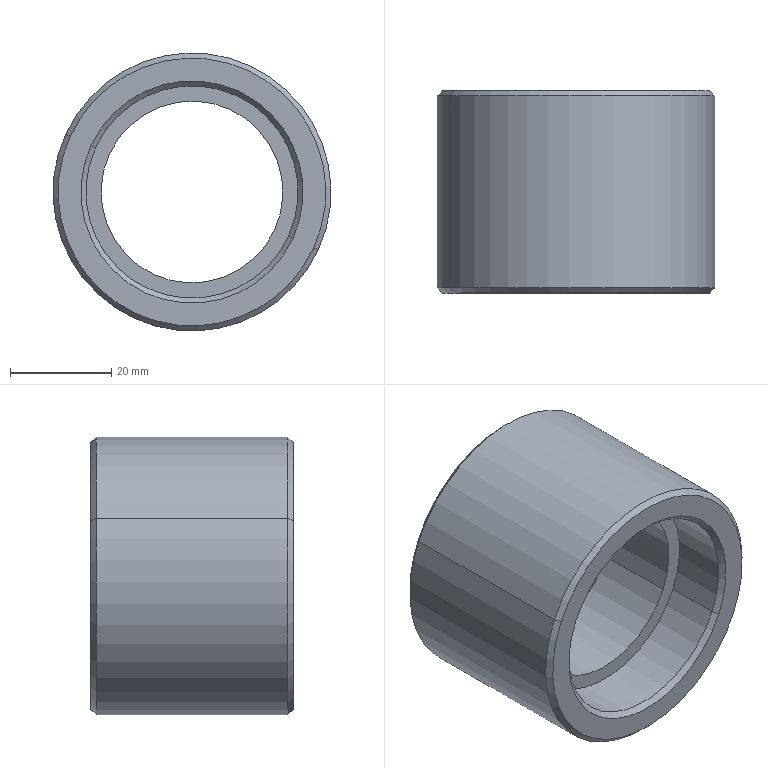Part | NX | features 0 2 | 1 solid | 20 faces | box 55 x 40 x 55 mm | volume 45192 mm3 | cone 8 | cylinder 8 | plane 4 | commonest cylinder face diameters 42 x4 36 x2 55 x2
STEP:
#1=CARTESIAN_POINT('',(19.105,99.,-276.846));
#2=VERTEX_POINT('',#1);
#3=CARTESIAN_POINT('',(-19.105,99.,-259.412));
#4=VERTEX_POINT('',#3);
#5=CARTESIAN_POINT('',(0.,99.,-268.129));
#6=DIRECTION('',(0.,-1.,0.));
#7=DIRECTION('',(0.9098,0.,-0.4151));
#8=AXIS2_PLACEMENT_3D('',#5,#6,#7);
#9=CIRCLE('',#8,21.);
#10=EDGE_CURVE('',#2,#4,#9,.T.);
#11=ORIENTED_EDGE('',*,*,#10,.T.);
#12=CARTESIAN_POINT('',(-20.015,100.,-258.997));
#13=VERTEX_POINT('',#12);
#14=CARTESIAN_POINT('',(-20.015,100.,-258.997));
#15=DIRECTION('',(0.6433,-0.7071,-0.2935));
#16=VECTOR('',#15,1000.);
#17=LINE('',#14,#16);
#18=EDGE_CURVE('',#13,#4,#17,.T.);
#19=ORIENTED_EDGE('',*,*,#18,.F.);
#20=CARTESIAN_POINT('',(20.015,100.,-277.261));
#21=VERTEX_POINT('',#20);
#22=CARTESIAN_POINT('',(0.,100.,-268.129));
#23=DIRECTION('',(0.,-1.,0.));
#24=DIRECTION('',(0.9098,0.,-0.4151));
#25=AXIS2_PLACEMENT_3D('',#22,#23,#24);
#26=CIRCLE('',#25,22.);
#27=EDGE_CURVE('',#21,#13,#26,.T.);
#28=ORIENTED_EDGE('',*,*,#27,.F.);
#29=CARTESIAN_POINT('',(20.015,100.,-277.261));
#30=DIRECTION('',(-0.6433,-0.7071,0.2935));
#31=VECTOR('',#30,1000.);
#32=LINE('',#29,#31);
#33=EDGE_CURVE('',#2,#21,#32,.F.);
#34=ORIENTED_EDGE('',*,*,#33,.F.);
#35=EDGE_LOOP('',(#11,#19,#28,#34));
#36=FACE_BOUND('',#35,.T.);
#37=CARTESIAN_POINT('',(0.,98.926,-268.129));
#38=DIRECTION('',(0.,1.,0.));
#39=DIRECTION('',(-0.9098,0.,0.4151));
#40=AXIS2_PLACEMENT_3D('',#37,#38,#39);
#41=CONICAL_SURFACE('',#40,20.926,0.7854);
#42=ADVANCED_FACE('',(#36),#41,.F.);
#43=ORIENTED_EDGE('',*,*,#33,.T.);
#44=CARTESIAN_POINT('',(0.,100.,-268.129));
#45=DIRECTION('',(0.,-1.,0.));
#46=DIRECTION('',(-0.9098,0.,0.4151));
#47=AXIS2_PLACEMENT_3D('',#44,#45,#46);
#48=CIRCLE('',#47,22.);
#49=EDGE_CURVE('',#13,#21,#48,.T.);
#50=ORIENTED_EDGE('',*,*,#49,.F.);
#51=ORIENTED_EDGE('',*,*,#18,.T.);
#52=CARTESIAN_POINT('',(0.,99.,-268.129));
#53=DIRECTION('',(0.,-1.,0.));
#54=DIRECTION('',(-0.9098,0.,0.4151));
#55=AXIS2_PLACEMENT_3D('',#52,#53,#54);
#56=CIRCLE('',#55,21.);
#57=EDGE_CURVE('',#4,#2,#56,.T.);
#58=ORIENTED_EDGE('',*,*,#57,.T.);
#59=EDGE_LOOP('',(#43,#50,#51,#58));
#60=FACE_BOUND('',#59,.T.);
#61=CARTESIAN_POINT('',(0.,98.926,-268.129));
#62=DIRECTION('',(0.,1.,0.));
#63=DIRECTION('',(-0.9098,0.,0.4151));
#64=AXIS2_PLACEMENT_3D('',#61,#62,#63);
#65=CONICAL_SURFACE('',#64,20.926,0.7854);
#66=ADVANCED_FACE('',(#60),#65,.F.);
#67=CARTESIAN_POINT('',(19.105,88.,-276.846));
#68=VERTEX_POINT('',#67);
#69=CARTESIAN_POINT('',(19.105,99.,-276.846));
#70=DIRECTION('',(0.,-1.,0.));
#71=VECTOR('',#70,1000.);
#72=LINE('',#69,#71);
#73=EDGE_CURVE('',#2,#68,#72,.T.);
#74=ORIENTED_EDGE('',*,*,#73,.F.);
#75=ORIENTED_EDGE('',*,*,#57,.F.);
#76=CARTESIAN_POINT('',(-19.105,88.,-259.412));
#77=VERTEX_POINT('',#76);
#78=CARTESIAN_POINT('',(-19.105,99.,-259.412));
#79=DIRECTION('',(0.,-1.,0.));
#80=VECTOR('',#79,1000.);
#81=LINE('',#78,#80);
#82=EDGE_CURVE('',#77,#4,#81,.F.);
#83=ORIENTED_EDGE('',*,*,#82,.F.);
#84=CARTESIAN_POINT('',(0.,88.,-268.129));
#85=DIRECTION('',(0.,1.,0.));
#86=DIRECTION('',(0.9098,0.,-0.4151));
#87=AXIS2_PLACEMENT_3D('',#84,#85,#86);
#88=CIRCLE('',#87,21.);
#89=EDGE_CURVE('',#68,#77,#88,.T.);
#90=ORIENTED_EDGE('',*,*,#89,.F.);
#91=EDGE_LOOP('',(#74,#75,#83,#90));
#92=FACE_BOUND('',#91,.T.);
#93=CARTESIAN_POINT('',(0.,88.,-268.129));
#94=DIRECTION('',(0.,1.,0.));
#95=DIRECTION('',(-0.9098,0.,0.4151));
#96=AXIS2_PLACEMENT_3D('',#93,#94,#95);
#97=CYLINDRICAL_SURFACE('',#96,21.);
#98=ADVANCED_FACE('',(#92),#97,.F.);
#99=CARTESIAN_POINT('',(0.,88.,-268.129));
#100=DIRECTION('',(0.,1.,0.));
#101=DIRECTION('',(-0.9098,0.,0.4151));
#102=AXIS2_PLACEMENT_3D('',#99,#100,#101);
#103=CIRCLE('',#102,21.);
#104=EDGE_CURVE('',#77,#68,#103,.T.);
#105=ORIENTED_EDGE('',*,*,#104,.F.);
#106=ORIENTED_EDGE('',*,*,#82,.T.);
#107=ORIENTED_EDGE('',*,*,#10,.F.);
#108=ORIENTED_EDGE('',*,*,#73,.T.);
#109=EDGE_LOOP('',(#105,#106,#107,#108));
#110=FACE_BOUND('',#109,.T.);
#111=CARTESIAN_POINT('',(0.,88.,-268.129));
#112=DIRECTION('',(0.,1.,0.));
#113=DIRECTION('',(-0.9098,0.,0.4151));
#114=AXIS2_PLACEMENT_3D('',#111,#112,#113);
#115=CYLINDRICAL_SURFACE('',#114,21.);
#116=ADVANCED_FACE('',(#110),#115,.F.);
#117=CARTESIAN_POINT('',(-16.376,88.,-260.658));
#118=VERTEX_POINT('',#117);
#119=CARTESIAN_POINT('',(16.376,88.,-275.601));
#120=VERTEX_POINT('',#119);
#121=CARTESIAN_POINT('',(0.,88.,-268.129));
#122=DIRECTION('',(0.,-1.,0.));
#123=DIRECTION('',(-0.9098,0.,0.4151));
#124=AXIS2_PLACEMENT_3D('',#121,#122,#123);
#125=CIRCLE('',#124,18.);
#126=EDGE_CURVE('',#118,#120,#125,.T.);
#127=ORIENTED_EDGE('',*,*,#126,.T.);
#128=CARTESIAN_POINT('',(0.,88.,-268.129));
#129=DIRECTION('',(0.,-1.,0.));
#130=DIRECTION('',(0.9098,0.,-0.4151));
#131=AXIS2_PLACEMENT_3D('',#128,#129,#130);
#132=CIRCLE('',#131,18.);
#133=EDGE_CURVE('',#120,#118,#132,.T.);
#134=ORIENTED_EDGE('',*,*,#133,.T.);
#135=EDGE_LOOP('',(#127,#134));
#136=FACE_BOUND('',#135,.T.);
#137=ORIENTED_EDGE('',*,*,#89,.T.);
#138=ORIENTED_EDGE('',*,*,#104,.T.);
#139=EDGE_LOOP('',(#137,#138));
#140=FACE_BOUND('',#139,.T.);
#141=CARTESIAN_POINT('',(0.,88.,-268.129));
#142=DIRECTION('',(0.,1.,0.));
#143=DIRECTION('',(-0.9098,0.,0.4151));
#144=AXIS2_PLACEMENT_3D('',#141,#142,#143);
#145=PLANE('',#144);
#146=ADVANCED_FACE('',(#136,#140),#145,.T.);
#147=CARTESIAN_POINT('',(-16.376,72.,-260.658));
#148=VERTEX_POINT('',#147);
#149=CARTESIAN_POINT('',(16.376,72.,-275.601));
#150=VERTEX_POINT('',#149);
#151=CARTESIAN_POINT('',(0.,72.,-268.129));
#152=DIRECTION('',(0.,1.,0.));
#153=DIRECTION('',(-0.9098,0.,0.4151));
#154=AXIS2_PLACEMENT_3D('',#151,#152,#153);
#155=CIRCLE('',#154,18.);
#156=EDGE_CURVE('',#148,#150,#155,.T.);
#157=ORIENTED_EDGE('',*,*,#156,.F.);
#158=CARTESIAN_POINT('',(-16.376,88.,-260.658));
#159=DIRECTION('',(0.,-1.,0.));
#160=VECTOR('',#159,1000.);
#161=LINE('',#158,#160);
#162=EDGE_CURVE('',#148,#118,#161,.F.);
#163=ORIENTED_EDGE('',*,*,#162,.T.);
#164=ORIENTED_EDGE('',*,*,#133,.F.);
#165=CARTESIAN_POINT('',(16.376,88.,-275.601));
#166=DIRECTION('',(0.,-1.,0.));
#167=VECTOR('',#166,1000.);
#168=LINE('',#165,#167);
#169=EDGE_CURVE('',#120,#150,#168,.T.);
#170=ORIENTED_EDGE('',*,*,#169,.T.);
#171=EDGE_LOOP('',(#157,#163,#164,#170));
#172=FACE_BOUND('',#171,.T.);
#173=CARTESIAN_POINT('',(0.,60.,-268.129));
#174=DIRECTION('',(0.,1.,0.));
#175=DIRECTION('',(-0.9098,0.,0.4151));
#176=AXIS2_PLACEMENT_3D('',#173,#174,#175);
#177=CYLINDRICAL_SURFACE('',#176,18.);
#178=ADVANCED_FACE('',(#172),#177,.F.);
#179=ORIENTED_EDGE('',*,*,#169,.F.);
#180=ORIENTED_EDGE('',*,*,#126,.F.);
#181=ORIENTED_EDGE('',*,*,#162,.F.);
#182=CARTESIAN_POINT('',(0.,72.,-268.129));
#183=DIRECTION('',(0.,1.,0.));
#184=DIRECTION('',(0.9098,0.,-0.4151));
#185=AXIS2_PLACEMENT_3D('',#182,#183,#184);
#186=CIRCLE('',#185,18.);
#187=EDGE_CURVE('',#150,#148,#186,.T.);
#188=ORIENTED_EDGE('',*,*,#187,.F.);
#189=EDGE_LOOP('',(#179,#180,#181,#188));
#190=FACE_BOUND('',#189,.T.);
#191=CARTESIAN_POINT('',(0.,60.,-268.129));
#192=DIRECTION('',(0.,1.,0.));
#193=DIRECTION('',(-0.9098,0.,0.4151));
#194=AXIS2_PLACEMENT_3D('',#191,#192,#193);
#195=CYLINDRICAL_SURFACE('',#194,18.);
#196=ADVANCED_FACE('',(#190),#195,.F.);
#197=CARTESIAN_POINT('',(-19.105,61.,-259.412));
#198=VERTEX_POINT('',#197);
#199=CARTESIAN_POINT('',(19.105,61.,-276.846));
#200=VERTEX_POINT('',#199);
#201=CARTESIAN_POINT('',(0.,61.,-268.129));
#202=DIRECTION('',(0.,1.,0.));
#203=DIRECTION('',(-0.9098,0.,0.4151));
#204=AXIS2_PLACEMENT_3D('',#201,#202,#203);
#205=CIRCLE('',#204,21.);
#206=EDGE_CURVE('',#198,#200,#205,.T.);
#207=ORIENTED_EDGE('',*,*,#206,.T.);
#208=CARTESIAN_POINT('',(20.015,60.,-277.261));
#209=VERTEX_POINT('',#208);
#210=CARTESIAN_POINT('',(20.015,60.,-277.261));
#211=DIRECTION('',(-0.6433,0.7071,0.2935));
#212=VECTOR('',#211,1000.);
#213=LINE('',#210,#212);
#214=EDGE_CURVE('',#209,#200,#213,.T.);
#215=ORIENTED_EDGE('',*,*,#214,.F.);
#216=CARTESIAN_POINT('',(-20.015,60.,-258.997));
#217=VERTEX_POINT('',#216);
#218=CARTESIAN_POINT('',(0.,60.,-268.129));
#219=DIRECTION('',(0.,1.,0.));
#220=DIRECTION('',(-0.9098,0.,0.4151));
#221=AXIS2_PLACEMENT_3D('',#218,#219,#220);
#222=CIRCLE('',#221,22.);
#223=EDGE_CURVE('',#217,#209,#222,.T.);
#224=ORIENTED_EDGE('',*,*,#223,.F.);
#225=CARTESIAN_POINT('',(-20.015,60.,-258.997));
#226=DIRECTION('',(0.6433,0.7071,-0.2935));
#227=VECTOR('',#226,1000.);
#228=LINE('',#225,#227);
#229=EDGE_CURVE('',#198,#217,#228,.F.);
#230=ORIENTED_EDGE('',*,*,#229,.F.);
#231=EDGE_LOOP('',(#207,#215,#224,#230));
#232=FACE_BOUND('',#231,.T.);
#233=CARTESIAN_POINT('',(0.,61.074,-268.129));
#234=DIRECTION('',(0.,-1.,0.));
#235=DIRECTION('',(0.9098,0.,-0.4151));
#236=AXIS2_PLACEMENT_3D('',#233,#234,#235);
#237=CONICAL_SURFACE('',#236,20.926,0.7854);
#238=ADVANCED_FACE('',(#232),#237,.F.);
#239=CARTESIAN_POINT('',(19.105,72.,-276.846));
#240=VERTEX_POINT('',#239);
#241=CARTESIAN_POINT('',(-19.105,72.,-259.412));
#242=VERTEX_POINT('',#241);
#243=CARTESIAN_POINT('',(0.,72.,-268.129));
#244=DIRECTION('',(0.,-1.,0.));
#245=DIRECTION('',(0.9098,0.,-0.4151));
#246=AXIS2_PLACEMENT_3D('',#243,#244,#245);
#247=CIRCLE('',#246,21.);
#248=EDGE_CURVE('',#240,#242,#247,.T.);
#249=ORIENTED_EDGE('',*,*,#248,.F.);
#250=CARTESIAN_POINT('',(19.105,61.,-276.846));
#251=DIRECTION('',(0.,1.,0.));
#252=VECTOR('',#251,1000.);
#253=LINE('',#250,#252);
#254=EDGE_CURVE('',#200,#240,#253,.T.);
#255=ORIENTED_EDGE('',*,*,#254,.F.);
#256=ORIENTED_EDGE('',*,*,#206,.F.);
#257=CARTESIAN_POINT('',(-19.105,61.,-259.412));
#258=DIRECTION('',(0.,1.,0.));
#259=VECTOR('',#258,1000.);
#260=LINE('',#257,#259);
#261=EDGE_CURVE('',#242,#198,#260,.F.);
#262=ORIENTED_EDGE('',*,*,#261,.F.);
#263=EDGE_LOOP('',(#249,#255,#256,#262));
#264=FACE_BOUND('',#263,.T.);
#265=CARTESIAN_POINT('',(0.,72.,-268.129));
#266=DIRECTION('',(0.,-1.,0.));
#267=DIRECTION('',(0.9098,0.,-0.4151));
#268=AXIS2_PLACEMENT_3D('',#265,#266,#267);
#269=CYLINDRICAL_SURFACE('',#268,21.);
#270=ADVANCED_FACE('',(#264),#269,.F.);
#271=ORIENTED_EDGE('',*,*,#156,.T.);
#272=ORIENTED_EDGE('',*,*,#187,.T.);
#273=EDGE_LOOP('',(#271,#272));
#274=FACE_BOUND('',#273,.T.);
#275=ORIENTED_EDGE('',*,*,#248,.T.);
#276=CARTESIAN_POINT('',(0.,72.,-268.129));
#277=DIRECTION('',(0.,-1.,0.));
#278=DIRECTION('',(-0.9098,0.,0.4151));
#279=AXIS2_PLACEMENT_3D('',#276,#277,#278);
#280=CIRCLE('',#279,21.);
#281=EDGE_CURVE('',#242,#240,#280,.T.);
#282=ORIENTED_EDGE('',*,*,#281,.T.);
#283=EDGE_LOOP('',(#275,#282));
#284=FACE_BOUND('',#283,.T.);
#285=CARTESIAN_POINT('',(0.,72.,-268.129));
#286=DIRECTION('',(0.,-1.,0.));
#287=DIRECTION('',(-0.9098,0.,0.4151));
#288=AXIS2_PLACEMENT_3D('',#285,#286,#287);
#289=PLANE('',#288);
#290=ADVANCED_FACE('',(#274,#284),#289,.T.);
#291=ORIENTED_EDGE('',*,*,#261,.T.);
#292=CARTESIAN_POINT('',(0.,61.,-268.129));
#293=DIRECTION('',(0.,1.,0.));
#294=DIRECTION('',(0.9098,0.,-0.4151));
#295=AXIS2_PLACEMENT_3D('',#292,#293,#294);
#296=CIRCLE('',#295,21.);
#297=EDGE_CURVE('',#200,#198,#296,.T.);
#298=ORIENTED_EDGE('',*,*,#297,.F.);
#299=ORIENTED_EDGE('',*,*,#254,.T.);
#300=ORIENTED_EDGE('',*,*,#281,.F.);
#301=EDGE_LOOP('',(#291,#298,#299,#300));
#302=FACE_BOUND('',#301,.T.);
#303=CARTESIAN_POINT('',(0.,72.,-268.129));
#304=DIRECTION('',(0.,-1.,0.));
#305=DIRECTION('',(0.9098,0.,-0.4151));
#306=AXIS2_PLACEMENT_3D('',#303,#304,#305);
#307=CYLINDRICAL_SURFACE('',#306,21.);
#308=ADVANCED_FACE('',(#302),#307,.F.);
#309=ORIENTED_EDGE('',*,*,#229,.T.);
#310=CARTESIAN_POINT('',(0.,60.,-268.129));
#311=DIRECTION('',(0.,1.,0.));
#312=DIRECTION('',(0.9098,0.,-0.4151));
#313=AXIS2_PLACEMENT_3D('',#310,#311,#312);
#314=CIRCLE('',#313,22.);
#315=EDGE_CURVE('',#209,#217,#314,.T.);
#316=ORIENTED_EDGE('',*,*,#315,.F.);
#317=ORIENTED_EDGE('',*,*,#214,.T.);
#318=ORIENTED_EDGE('',*,*,#297,.T.);
#319=EDGE_LOOP('',(#309,#316,#317,#318));
#320=FACE_BOUND('',#319,.T.);
#321=CARTESIAN_POINT('',(0.,61.074,-268.129));
#322=DIRECTION('',(0.,-1.,0.));
#323=DIRECTION('',(0.9098,0.,-0.4151));
#324=AXIS2_PLACEMENT_3D('',#321,#322,#323);
#325=CONICAL_SURFACE('',#324,20.926,0.7854);
#326=ADVANCED_FACE('',(#320),#325,.F.);
#327=CARTESIAN_POINT('',(-24.109,60.,-257.129));
#328=VERTEX_POINT('',#327);
#329=CARTESIAN_POINT('',(24.109,60.,-279.129));
#330=VERTEX_POINT('',#329);
#331=CARTESIAN_POINT('',(0.,60.,-268.129));
#332=DIRECTION('',(0.,-1.,0.));
#333=DIRECTION('',(-0.9098,0.,0.4151));
#334=AXIS2_PLACEMENT_3D('',#331,#332,#333);
#335=CIRCLE('',#334,26.5);
#336=EDGE_CURVE('',#328,#330,#335,.T.);
#337=ORIENTED_EDGE('',*,*,#336,.F.);
#338=CARTESIAN_POINT('',(-25.019,61.,-256.714));
#339=VERTEX_POINT('',#338);
#340=CARTESIAN_POINT('',(-25.019,61.,-256.714));
#341=DIRECTION('',(0.6433,-0.7071,-0.2935));
#342=VECTOR('',#341,1000.);
#343=LINE('',#340,#342);
#344=EDGE_CURVE('',#328,#339,#343,.F.);
#345=ORIENTED_EDGE('',*,*,#344,.T.);
#346=CARTESIAN_POINT('',(25.019,61.,-279.545));
#347=VERTEX_POINT('',#346);
#348=CARTESIAN_POINT('',(0.,61.,-268.129));
#349=DIRECTION('',(0.,-1.,0.));
#350=DIRECTION('',(-0.9098,0.,0.4151));
#351=AXIS2_PLACEMENT_3D('',#348,#349,#350);
#352=CIRCLE('',#351,27.5);
#353=EDGE_CURVE('',#339,#347,#352,.T.);
#354=ORIENTED_EDGE('',*,*,#353,.T.);
#355=CARTESIAN_POINT('',(25.019,61.,-279.545));
#356=DIRECTION('',(-0.6433,-0.7071,0.2935));
#357=VECTOR('',#356,1000.);
#358=LINE('',#355,#357);
#359=EDGE_CURVE('',#347,#330,#358,.T.);
#360=ORIENTED_EDGE('',*,*,#359,.T.);
#361=EDGE_LOOP('',(#337,#345,#354,#360));
#362=FACE_BOUND('',#361,.T.);
#363=CARTESIAN_POINT('',(0.,59.926,-268.129));
#364=DIRECTION('',(0.,1.,0.));
#365=DIRECTION('',(-0.9098,0.,0.4151));
#366=AXIS2_PLACEMENT_3D('',#363,#364,#365);
#367=CONICAL_SURFACE('',#366,26.426,0.7854);
#368=ADVANCED_FACE('',(#362),#367,.T.);
#369=ORIENTED_EDGE('',*,*,#223,.T.);
#370=ORIENTED_EDGE('',*,*,#315,.T.);
#371=EDGE_LOOP('',(#369,#370));
#372=FACE_BOUND('',#371,.T.);
#373=CARTESIAN_POINT('',(0.,60.,-268.129));
#374=DIRECTION('',(0.,-1.,0.));
#375=DIRECTION('',(0.9098,0.,-0.4151));
#376=AXIS2_PLACEMENT_3D('',#373,#374,#375);
#377=CIRCLE('',#376,26.5);
#378=EDGE_CURVE('',#330,#328,#377,.T.);
#379=ORIENTED_EDGE('',*,*,#378,.T.);
#380=ORIENTED_EDGE('',*,*,#336,.T.);
#381=EDGE_LOOP('',(#379,#380));
#382=FACE_BOUND('',#381,.T.);
#383=CARTESIAN_POINT('',(0.,60.,-268.129));
#384=DIRECTION('',(0.,1.,0.));
#385=DIRECTION('',(-0.9098,0.,0.4151));
#386=AXIS2_PLACEMENT_3D('',#383,#384,#385);
#387=PLANE('',#386);
#388=ADVANCED_FACE('',(#372,#382),#387,.F.);
#389=ORIENTED_EDGE('',*,*,#359,.F.);
#390=CARTESIAN_POINT('',(0.,61.,-268.129));
#391=DIRECTION('',(0.,-1.,0.));
#392=DIRECTION('',(0.9098,0.,-0.4151));
#393=AXIS2_PLACEMENT_3D('',#390,#391,#392);
#394=CIRCLE('',#393,27.5);
#395=EDGE_CURVE('',#347,#339,#394,.T.);
#396=ORIENTED_EDGE('',*,*,#395,.T.);
#397=ORIENTED_EDGE('',*,*,#344,.F.);
#398=ORIENTED_EDGE('',*,*,#378,.F.);
#399=EDGE_LOOP('',(#389,#396,#397,#398));
#400=FACE_BOUND('',#399,.T.);
#401=CARTESIAN_POINT('',(0.,59.926,-268.129));
#402=DIRECTION('',(0.,1.,0.));
#403=DIRECTION('',(-0.9098,0.,0.4151));
#404=AXIS2_PLACEMENT_3D('',#401,#402,#403);
#405=CONICAL_SURFACE('',#404,26.426,0.7854);
#406=ADVANCED_FACE('',(#400),#405,.T.);
#407=CARTESIAN_POINT('',(-25.019,99.,-256.714));
#408=VERTEX_POINT('',#407);
#409=CARTESIAN_POINT('',(-25.019,61.,-256.714));
#410=DIRECTION('',(0.,1.,0.));
#411=VECTOR('',#410,1000.);
#412=LINE('',#409,#411);
#413=EDGE_CURVE('',#408,#339,#412,.F.);
#414=ORIENTED_EDGE('',*,*,#413,.T.);
#415=ORIENTED_EDGE('',*,*,#395,.F.);
#416=CARTESIAN_POINT('',(25.019,99.,-279.545));
#417=VERTEX_POINT('',#416);
#418=CARTESIAN_POINT('',(25.019,61.,-279.545));
#419=DIRECTION('',(0.,1.,0.));
#420=VECTOR('',#419,1000.);
#421=LINE('',#418,#420);
#422=EDGE_CURVE('',#347,#417,#421,.T.);
#423=ORIENTED_EDGE('',*,*,#422,.T.);
#424=CARTESIAN_POINT('',(0.,99.,-268.129));
#425=DIRECTION('',(0.,1.,0.));
#426=DIRECTION('',(-0.9098,0.,0.4151));
#427=AXIS2_PLACEMENT_3D('',#424,#425,#426);
#428=CIRCLE('',#427,27.5);
#429=EDGE_CURVE('',#408,#417,#428,.T.);
#430=ORIENTED_EDGE('',*,*,#429,.F.);
#431=EDGE_LOOP('',(#414,#415,#423,#430));
#432=FACE_BOUND('',#431,.T.);
#433=CARTESIAN_POINT('',(0.,100.,-268.129));
#434=DIRECTION('',(0.,-1.,0.));
#435=DIRECTION('',(0.9098,0.,-0.4151));
#436=AXIS2_PLACEMENT_3D('',#433,#434,#435);
#437=CYLINDRICAL_SURFACE('',#436,27.5);
#438=ADVANCED_FACE('',(#432),#437,.T.);
#439=CARTESIAN_POINT('',(0.,99.,-268.129));
#440=DIRECTION('',(0.,1.,0.));
#441=DIRECTION('',(0.9098,0.,-0.4151));
#442=AXIS2_PLACEMENT_3D('',#439,#440,#441);
#443=CIRCLE('',#442,27.5);
#444=EDGE_CURVE('',#417,#408,#443,.T.);
#445=ORIENTED_EDGE('',*,*,#444,.F.);
#446=ORIENTED_EDGE('',*,*,#422,.F.);
#447=ORIENTED_EDGE('',*,*,#353,.F.);
#448=ORIENTED_EDGE('',*,*,#413,.F.);
#449=EDGE_LOOP('',(#445,#446,#447,#448));
#450=FACE_BOUND('',#449,.T.);
#451=CARTESIAN_POINT('',(0.,100.,-268.129));
#452=DIRECTION('',(0.,-1.,0.));
#453=DIRECTION('',(0.9098,0.,-0.4151));
#454=AXIS2_PLACEMENT_3D('',#451,#452,#453);
#455=CYLINDRICAL_SURFACE('',#454,27.5);
#456=ADVANCED_FACE('',(#450),#455,.T.);
#457=CARTESIAN_POINT('',(24.109,100.,-279.129));
#458=VERTEX_POINT('',#457);
#459=CARTESIAN_POINT('',(-24.109,100.,-257.129));
#460=VERTEX_POINT('',#459);
#461=CARTESIAN_POINT('',(0.,100.,-268.129));
#462=DIRECTION('',(0.,1.,0.));
#463=DIRECTION('',(0.9098,0.,-0.4151));
#464=AXIS2_PLACEMENT_3D('',#461,#462,#463);
#465=CIRCLE('',#464,26.5);
#466=EDGE_CURVE('',#458,#460,#465,.T.);
#467=ORIENTED_EDGE('',*,*,#466,.F.);
#468=CARTESIAN_POINT('',(25.019,99.,-279.545));
#469=DIRECTION('',(-0.6433,0.7071,0.2935));
#470=VECTOR('',#469,1000.);
#471=LINE('',#468,#470);
#472=EDGE_CURVE('',#458,#417,#471,.F.);
#473=ORIENTED_EDGE('',*,*,#472,.T.);
#474=ORIENTED_EDGE('',*,*,#444,.T.);
#475=CARTESIAN_POINT('',(-25.019,99.,-256.714));
#476=DIRECTION('',(0.6433,0.7071,-0.2935));
#477=VECTOR('',#476,1000.);
#478=LINE('',#475,#477);
#479=EDGE_CURVE('',#408,#460,#478,.T.);
#480=ORIENTED_EDGE('',*,*,#479,.T.);
#481=EDGE_LOOP('',(#467,#473,#474,#480));
#482=FACE_BOUND('',#481,.T.);
#483=CARTESIAN_POINT('',(0.,100.074,-268.129));
#484=DIRECTION('',(0.,-1.,0.));
#485=DIRECTION('',(0.9098,0.,-0.4151));
#486=AXIS2_PLACEMENT_3D('',#483,#484,#485);
#487=CONICAL_SURFACE('',#486,26.426,0.7854);
#488=ADVANCED_FACE('',(#482),#487,.T.);
#489=ORIENTED_EDGE('',*,*,#27,.T.);
#490=ORIENTED_EDGE('',*,*,#49,.T.);
#491=EDGE_LOOP('',(#489,#490));
#492=FACE_BOUND('',#491,.T.);
#493=CARTESIAN_POINT('',(0.,100.,-268.129));
#494=DIRECTION('',(0.,1.,0.));
#495=DIRECTION('',(-0.9098,0.,0.4151));
#496=AXIS2_PLACEMENT_3D('',#493,#494,#495);
#497=CIRCLE('',#496,26.5);
#498=EDGE_CURVE('',#460,#458,#497,.T.);
#499=ORIENTED_EDGE('',*,*,#498,.T.);
#500=ORIENTED_EDGE('',*,*,#466,.T.);
#501=EDGE_LOOP('',(#499,#500));
#502=FACE_BOUND('',#501,.T.);
#503=CARTESIAN_POINT('',(0.,100.,-268.129));
#504=DIRECTION('',(0.,1.,0.));
#505=DIRECTION('',(-0.9098,0.,0.4151));
#506=AXIS2_PLACEMENT_3D('',#503,#504,#505);
#507=PLANE('',#506);
#508=ADVANCED_FACE('',(#492,#502),#507,.T.);
#509=ORIENTED_EDGE('',*,*,#479,.F.);
#510=ORIENTED_EDGE('',*,*,#429,.T.);
#511=ORIENTED_EDGE('',*,*,#472,.F.);
#512=ORIENTED_EDGE('',*,*,#498,.F.);
#513=EDGE_LOOP('',(#509,#510,#511,#512));
#514=FACE_BOUND('',#513,.T.);
#515=CARTESIAN_POINT('',(0.,100.074,-268.129));
#516=DIRECTION('',(0.,-1.,0.));
#517=DIRECTION('',(0.9098,0.,-0.4151));
#518=AXIS2_PLACEMENT_3D('',#515,#516,#517);
#519=CONICAL_SURFACE('',#518,26.426,0.7854);
#520=ADVANCED_FACE('',(#514),#519,.T.);
#521=CLOSED_SHELL('',(#42,#66,#98,#116,#146,#178,#196,#238,#270,#290,#308,#326,#368,#388,#406,#438,#456,#488,#508,#520));
#522=MANIFOLD_SOLID_BREP('',#521);
#523=(LENGTH_UNIT()NAMED_UNIT(*)SI_UNIT(.MILLI.,.METRE.));
#524=UNCERTAINTY_MEASURE_WITH_UNIT(LENGTH_MEASURE(0.00001),#523,'','');
#525=(NAMED_UNIT(*)PLANE_ANGLE_UNIT()SI_UNIT($,.RADIAN.));
#526=(NAMED_UNIT(*)SI_UNIT($,.STERADIAN.)SOLID_ANGLE_UNIT());
#527=(GEOMETRIC_REPRESENTATION_CONTEXT(3)GLOBAL_UNCERTAINTY_ASSIGNED_CONTEXT((#524))GLOBAL_UNIT_ASSIGNED_CONTEXT((#523,#525,#526))REPRESENTATION_CONTEXT('',''));
#528=ADVANCED_BREP_SHAPE_REPRESENTATION('',(#522),#527);